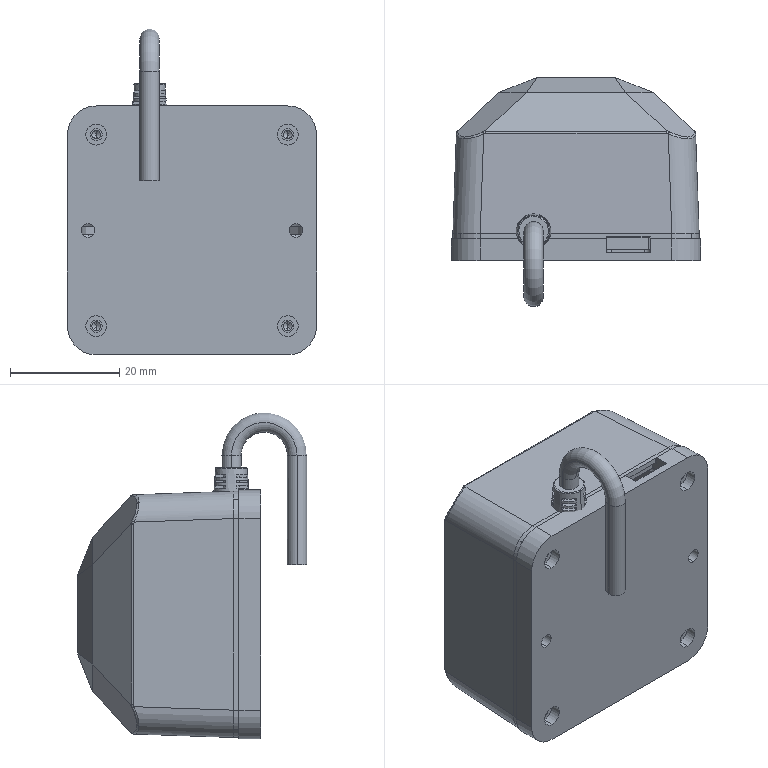Part | SolidWorks | features BaseBody 3, 3DProfileFeature 2, ICE 1, MoveCopyBody 1, NetBlend 1, RefAxis 1, Revolution 1, Sweep 1 | 3 solids | 545 faces | box 45.5 x 41.918 x 59.598 mm | volume 18797 mm3 | plane 316 | cylinder 154 | spline 53 | cone 19 | torus 3 | commonest cylinder face diameters 2 x28 3.535 x18 1 x12 1.6 x12 3 x12 5 x12